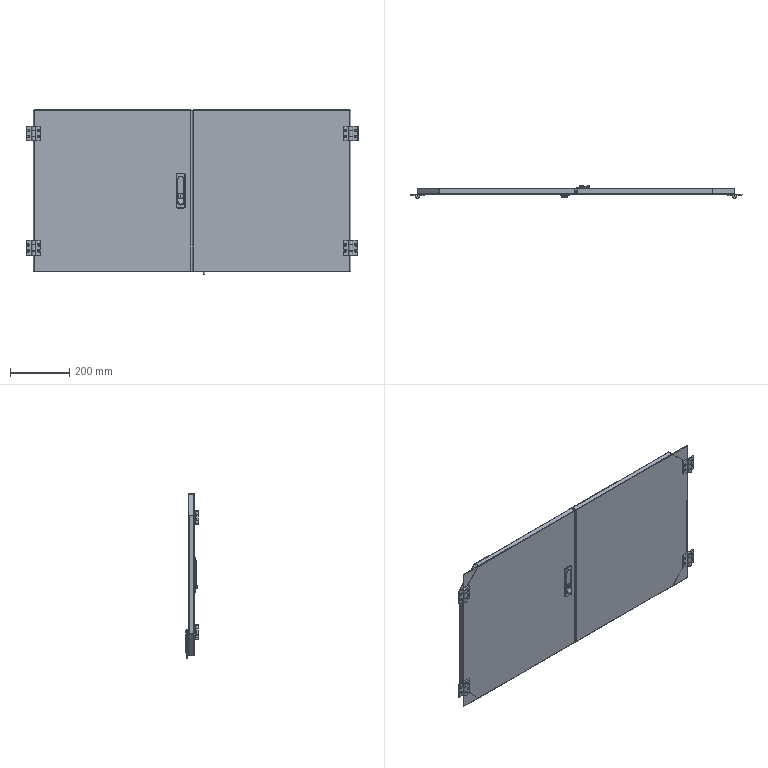Part | NX | features BREP 11 | 23 solids | 597 faces | box 1120 x 43.2 x 557.003 mm | volume 1208826 mm3 | plane 272 | cylinder 221 | sphere 40 | cone 34 | torus 22 | spline 8 | commonest cylinder face diameters 6 x54 4.4 x32 2 x23 3 x16 5 x16 10 x16